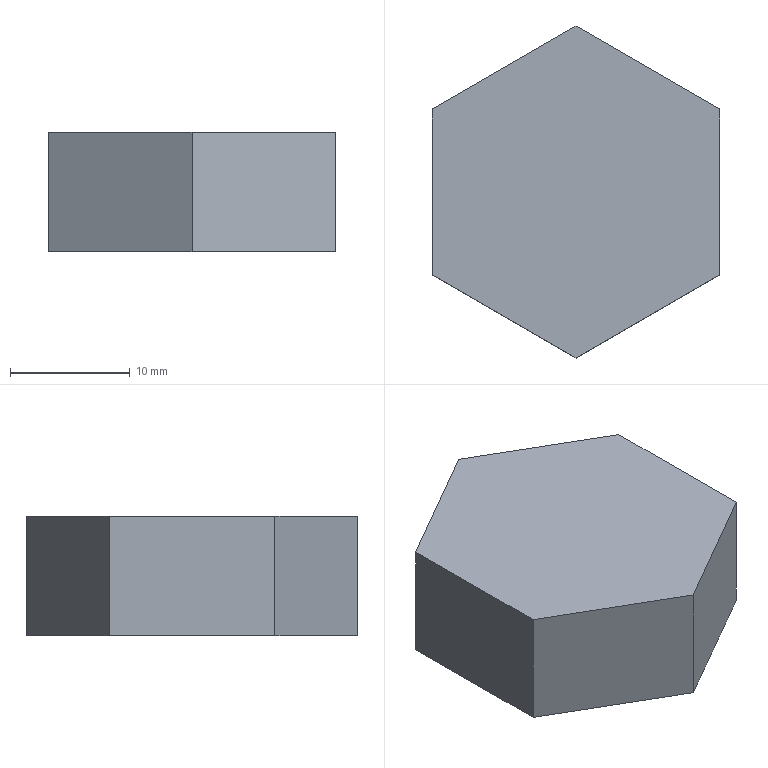Part | NX | features solid 2 | 1 solid | 8 faces | box 24 x 27.713 x 10 mm | volume 4988 mm3 | plane 8
STEP:
#1=CARTESIAN_POINT('',(267.,-16.928,-47.));
#2=VERTEX_POINT('',#1);
#3=CARTESIAN_POINT('',(255.,-23.856,-47.));
#4=VERTEX_POINT('',#3);
#5=CARTESIAN_POINT('',(267.,-16.928,-47.));
#6=DIRECTION('',(-0.866,-0.5,0.));
#7=VECTOR('',#6,1000.);
#8=LINE('',#5,#7);
#9=EDGE_CURVE('',#2,#4,#8,.T.);
#10=ORIENTED_EDGE('',*,*,#9,.F.);
#11=CARTESIAN_POINT('',(267.,-16.928,-37.));
#12=VERTEX_POINT('',#11);
#13=CARTESIAN_POINT('',(267.,-16.928,-37.));
#14=DIRECTION('',(0.,0.,-1.));
#15=VECTOR('',#14,1000.);
#16=LINE('',#13,#15);
#17=EDGE_CURVE('',#12,#2,#16,.T.);
#18=ORIENTED_EDGE('',*,*,#17,.F.);
#19=CARTESIAN_POINT('',(255.,-23.856,-37.));
#20=VERTEX_POINT('',#19);
#21=CARTESIAN_POINT('',(267.,-16.928,-37.));
#22=DIRECTION('',(-0.866,-0.5,0.));
#23=VECTOR('',#22,1000.);
#24=LINE('',#21,#23);
#25=EDGE_CURVE('',#12,#20,#24,.T.);
#26=ORIENTED_EDGE('',*,*,#25,.T.);
#27=CARTESIAN_POINT('',(255.,-23.856,-37.));
#28=DIRECTION('',(0.,0.,-1.));
#29=VECTOR('',#28,1000.);
#30=LINE('',#27,#29);
#31=EDGE_CURVE('',#20,#4,#30,.T.);
#32=ORIENTED_EDGE('',*,*,#31,.T.);
#33=EDGE_LOOP('',(#10,#18,#26,#32));
#34=FACE_BOUND('',#33,.T.);
#35=CARTESIAN_POINT('',(267.,-16.928,-37.));
#36=DIRECTION('',(0.5,-0.866,0.));
#37=DIRECTION('',(0.866,0.5,0.));
#38=AXIS2_PLACEMENT_3D('',#35,#36,#37);
#39=PLANE('',#38);
#40=ADVANCED_FACE('',(#34),#39,.T.);
#41=CARTESIAN_POINT('',(243.,-16.928,-47.));
#42=VERTEX_POINT('',#41);
#43=CARTESIAN_POINT('',(255.,-23.856,-47.));
#44=DIRECTION('',(-0.866,0.5,0.));
#45=VECTOR('',#44,1000.);
#46=LINE('',#43,#45);
#47=EDGE_CURVE('',#4,#42,#46,.T.);
#48=ORIENTED_EDGE('',*,*,#47,.F.);
#49=ORIENTED_EDGE('',*,*,#31,.F.);
#50=CARTESIAN_POINT('',(243.,-16.928,-37.));
#51=VERTEX_POINT('',#50);
#52=CARTESIAN_POINT('',(255.,-23.856,-37.));
#53=DIRECTION('',(-0.866,0.5,0.));
#54=VECTOR('',#53,1000.);
#55=LINE('',#52,#54);
#56=EDGE_CURVE('',#20,#51,#55,.T.);
#57=ORIENTED_EDGE('',*,*,#56,.T.);
#58=CARTESIAN_POINT('',(243.,-16.928,-37.));
#59=DIRECTION('',(0.,0.,-1.));
#60=VECTOR('',#59,1000.);
#61=LINE('',#58,#60);
#62=EDGE_CURVE('',#51,#42,#61,.T.);
#63=ORIENTED_EDGE('',*,*,#62,.T.);
#64=EDGE_LOOP('',(#48,#49,#57,#63));
#65=FACE_BOUND('',#64,.T.);
#66=CARTESIAN_POINT('',(255.,-23.856,-37.));
#67=DIRECTION('',(-0.5,-0.866,0.));
#68=DIRECTION('',(0.866,-0.5,0.));
#69=AXIS2_PLACEMENT_3D('',#66,#67,#68);
#70=PLANE('',#69);
#71=ADVANCED_FACE('',(#65),#70,.T.);
#72=CARTESIAN_POINT('',(243.,-3.072,-47.));
#73=VERTEX_POINT('',#72);
#74=CARTESIAN_POINT('',(243.,-16.928,-47.));
#75=DIRECTION('',(0.,1.,0.));
#76=VECTOR('',#75,1000.);
#77=LINE('',#74,#76);
#78=EDGE_CURVE('',#42,#73,#77,.T.);
#79=ORIENTED_EDGE('',*,*,#78,.F.);
#80=ORIENTED_EDGE('',*,*,#62,.F.);
#81=CARTESIAN_POINT('',(243.,-3.072,-37.));
#82=VERTEX_POINT('',#81);
#83=CARTESIAN_POINT('',(243.,-16.928,-37.));
#84=DIRECTION('',(0.,1.,0.));
#85=VECTOR('',#84,1000.);
#86=LINE('',#83,#85);
#87=EDGE_CURVE('',#51,#82,#86,.T.);
#88=ORIENTED_EDGE('',*,*,#87,.T.);
#89=CARTESIAN_POINT('',(243.,-3.072,-37.));
#90=DIRECTION('',(0.,0.,-1.));
#91=VECTOR('',#90,1000.);
#92=LINE('',#89,#91);
#93=EDGE_CURVE('',#82,#73,#92,.T.);
#94=ORIENTED_EDGE('',*,*,#93,.T.);
#95=EDGE_LOOP('',(#79,#80,#88,#94));
#96=FACE_BOUND('',#95,.T.);
#97=CARTESIAN_POINT('',(243.,-16.928,-37.));
#98=DIRECTION('',(-1.,0.,0.));
#99=DIRECTION('',(0.,-1.,0.));
#100=AXIS2_PLACEMENT_3D('',#97,#98,#99);
#101=PLANE('',#100);
#102=ADVANCED_FACE('',(#96),#101,.T.);
#103=CARTESIAN_POINT('',(255.,3.856,-47.));
#104=VERTEX_POINT('',#103);
#105=CARTESIAN_POINT('',(243.,-3.072,-47.));
#106=DIRECTION('',(0.866,0.5,0.));
#107=VECTOR('',#106,1000.);
#108=LINE('',#105,#107);
#109=EDGE_CURVE('',#73,#104,#108,.T.);
#110=ORIENTED_EDGE('',*,*,#109,.F.);
#111=ORIENTED_EDGE('',*,*,#93,.F.);
#112=CARTESIAN_POINT('',(255.,3.856,-37.));
#113=VERTEX_POINT('',#112);
#114=CARTESIAN_POINT('',(243.,-3.072,-37.));
#115=DIRECTION('',(0.866,0.5,0.));
#116=VECTOR('',#115,1000.);
#117=LINE('',#114,#116);
#118=EDGE_CURVE('',#82,#113,#117,.T.);
#119=ORIENTED_EDGE('',*,*,#118,.T.);
#120=CARTESIAN_POINT('',(255.,3.856,-37.));
#121=DIRECTION('',(0.,0.,-1.));
#122=VECTOR('',#121,1000.);
#123=LINE('',#120,#122);
#124=EDGE_CURVE('',#113,#104,#123,.T.);
#125=ORIENTED_EDGE('',*,*,#124,.T.);
#126=EDGE_LOOP('',(#110,#111,#119,#125));
#127=FACE_BOUND('',#126,.T.);
#128=CARTESIAN_POINT('',(243.,-3.072,-37.));
#129=DIRECTION('',(-0.5,0.866,0.));
#130=DIRECTION('',(-0.866,-0.5,0.));
#131=AXIS2_PLACEMENT_3D('',#128,#129,#130);
#132=PLANE('',#131);
#133=ADVANCED_FACE('',(#127),#132,.T.);
#134=CARTESIAN_POINT('',(267.,-3.072,-47.));
#135=VERTEX_POINT('',#134);
#136=CARTESIAN_POINT('',(255.,3.856,-47.));
#137=DIRECTION('',(0.866,-0.5,0.));
#138=VECTOR('',#137,1000.);
#139=LINE('',#136,#138);
#140=EDGE_CURVE('',#104,#135,#139,.T.);
#141=ORIENTED_EDGE('',*,*,#140,.F.);
#142=ORIENTED_EDGE('',*,*,#124,.F.);
#143=CARTESIAN_POINT('',(267.,-3.072,-37.));
#144=VERTEX_POINT('',#143);
#145=CARTESIAN_POINT('',(255.,3.856,-37.));
#146=DIRECTION('',(0.866,-0.5,0.));
#147=VECTOR('',#146,1000.);
#148=LINE('',#145,#147);
#149=EDGE_CURVE('',#113,#144,#148,.T.);
#150=ORIENTED_EDGE('',*,*,#149,.T.);
#151=CARTESIAN_POINT('',(267.,-3.072,-37.));
#152=DIRECTION('',(0.,0.,-1.));
#153=VECTOR('',#152,1000.);
#154=LINE('',#151,#153);
#155=EDGE_CURVE('',#144,#135,#154,.T.);
#156=ORIENTED_EDGE('',*,*,#155,.T.);
#157=EDGE_LOOP('',(#141,#142,#150,#156));
#158=FACE_BOUND('',#157,.T.);
#159=CARTESIAN_POINT('',(255.,3.856,-37.));
#160=DIRECTION('',(0.5,0.866,0.));
#161=DIRECTION('',(-0.866,0.5,0.));
#162=AXIS2_PLACEMENT_3D('',#159,#160,#161);
#163=PLANE('',#162);
#164=ADVANCED_FACE('',(#158),#163,.T.);
#165=CARTESIAN_POINT('',(267.,-3.072,-47.));
#166=DIRECTION('',(0.,-1.,0.));
#167=VECTOR('',#166,1000.);
#168=LINE('',#165,#167);
#169=EDGE_CURVE('',#135,#2,#168,.T.);
#170=ORIENTED_EDGE('',*,*,#169,.F.);
#171=ORIENTED_EDGE('',*,*,#155,.F.);
#172=CARTESIAN_POINT('',(267.,-3.072,-37.));
#173=DIRECTION('',(0.,-1.,0.));
#174=VECTOR('',#173,1000.);
#175=LINE('',#172,#174);
#176=EDGE_CURVE('',#144,#12,#175,.T.);
#177=ORIENTED_EDGE('',*,*,#176,.T.);
#178=ORIENTED_EDGE('',*,*,#17,.T.);
#179=EDGE_LOOP('',(#170,#171,#177,#178));
#180=FACE_BOUND('',#179,.T.);
#181=CARTESIAN_POINT('',(267.,-3.072,-37.));
#182=DIRECTION('',(1.,0.,0.));
#183=DIRECTION('',(0.,1.,0.));
#184=AXIS2_PLACEMENT_3D('',#181,#182,#183);
#185=PLANE('',#184);
#186=ADVANCED_FACE('',(#180),#185,.T.);
#187=ORIENTED_EDGE('',*,*,#25,.F.);
#188=ORIENTED_EDGE('',*,*,#176,.F.);
#189=ORIENTED_EDGE('',*,*,#149,.F.);
#190=ORIENTED_EDGE('',*,*,#118,.F.);
#191=ORIENTED_EDGE('',*,*,#87,.F.);
#192=ORIENTED_EDGE('',*,*,#56,.F.);
#193=EDGE_LOOP('',(#187,#188,#189,#190,#191,#192));
#194=FACE_BOUND('',#193,.T.);
#195=CARTESIAN_POINT('',(243.,-30.785,-37.));
#196=DIRECTION('',(0.,0.,-1.));
#197=DIRECTION('',(0.,-1.,0.));
#198=AXIS2_PLACEMENT_3D('',#195,#196,#197);
#199=PLANE('',#198);
#200=ADVANCED_FACE('',(#194),#199,.F.);
#201=ORIENTED_EDGE('',*,*,#9,.T.);
#202=ORIENTED_EDGE('',*,*,#47,.T.);
#203=ORIENTED_EDGE('',*,*,#78,.T.);
#204=ORIENTED_EDGE('',*,*,#109,.T.);
#205=ORIENTED_EDGE('',*,*,#140,.T.);
#206=ORIENTED_EDGE('',*,*,#169,.T.);
#207=EDGE_LOOP('',(#201,#202,#203,#204,#205,#206));
#208=FACE_BOUND('',#207,.T.);
#209=CARTESIAN_POINT('',(243.,-30.785,-47.));
#210=DIRECTION('',(0.,0.,-1.));
#211=DIRECTION('',(0.,-1.,0.));
#212=AXIS2_PLACEMENT_3D('',#209,#210,#211);
#213=PLANE('',#212);
#214=ADVANCED_FACE('',(#208),#213,.T.);
#215=CLOSED_SHELL('',(#40,#71,#102,#133,#164,#186,#200,#214));
#216=MANIFOLD_SOLID_BREP('',#215);
#217=(LENGTH_UNIT()NAMED_UNIT(*)SI_UNIT(.MILLI.,.METRE.));
#218=UNCERTAINTY_MEASURE_WITH_UNIT(LENGTH_MEASURE(0.00001),#217,'','');
#219=(NAMED_UNIT(*)PLANE_ANGLE_UNIT()SI_UNIT($,.RADIAN.));
#220=(NAMED_UNIT(*)SI_UNIT($,.STERADIAN.)SOLID_ANGLE_UNIT());
#221=(GEOMETRIC_REPRESENTATION_CONTEXT(3)GLOBAL_UNCERTAINTY_ASSIGNED_CONTEXT((#218))GLOBAL_UNIT_ASSIGNED_CONTEXT((#217,#219,#220))REPRESENTATION_CONTEXT('',''));
#222=ADVANCED_BREP_SHAPE_REPRESENTATION('',(#216),#221);